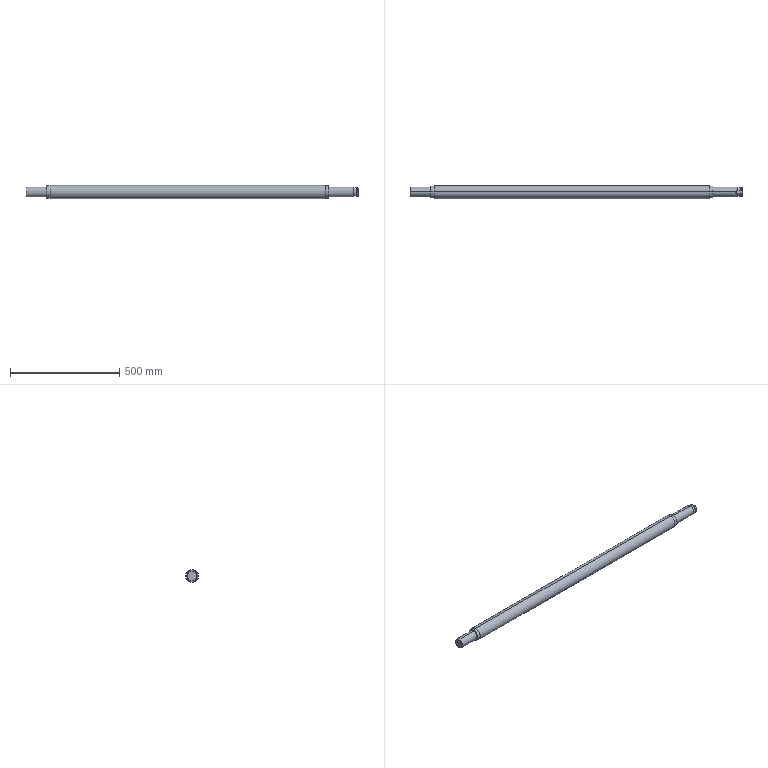Part | SolidWorks | features BaseBody 1 | 1 solid | 33 faces | box 1520 x 60 x 60 mm | volume 3990554 mm3 | cylinder 16 | plane 13 | cone 4 | commonest cylinder face diameters 45 x4 55 x4 12 x2 40 x2 60 x2 36 x1
STEP:
#1=CARTESIAN_POINT('',(3106.374,1848.107,21.685));
#2=VERTEX_POINT('',#1);
#3=CARTESIAN_POINT('',(3100.374,1842.107,22.5));
#4=VERTEX_POINT('',#3);
#5=CARTESIAN_POINT('',(3106.374,1848.107,21.685));
#6=CARTESIAN_POINT('',(3105.976,1848.107,21.685));
#7=CARTESIAN_POINT('',(3105.584,1848.068,21.696));
#8=CARTESIAN_POINT('',(3105.007,1847.953,21.727));
#9=CARTESIAN_POINT('',(3104.816,1847.905,21.74));
#10=CARTESIAN_POINT('',(3104.438,1847.79,21.771));
#11=CARTESIAN_POINT('',(3104.251,1847.723,21.788));
#12=CARTESIAN_POINT('',(3103.707,1847.496,21.846));
#13=CARTESIAN_POINT('',(3103.363,1847.312,21.891));
#14=CARTESIAN_POINT('',(3102.875,1846.985,21.965));
#15=CARTESIAN_POINT('',(3102.716,1846.867,21.991));
#16=CARTESIAN_POINT('',(3102.412,1846.617,22.044));
#17=CARTESIAN_POINT('',(3102.267,1846.486,22.07));
#18=CARTESIAN_POINT('',(3101.854,1846.073,22.15));
#19=CARTESIAN_POINT('',(3101.607,1845.772,22.202));
#20=CARTESIAN_POINT('',(3101.168,1845.116,22.3));
#21=CARTESIAN_POINT('',(3100.983,1844.769,22.345));
#22=CARTESIAN_POINT('',(3100.758,1844.228,22.401));
#23=CARTESIAN_POINT('',(3100.692,1844.044,22.417));
#24=CARTESIAN_POINT('',(3100.577,1843.667,22.447));
#25=CARTESIAN_POINT('',(3100.528,1843.473,22.459));
#26=CARTESIAN_POINT('',(3100.413,1842.892,22.49));
#27=CARTESIAN_POINT('',(3100.374,1842.501,22.5));
#28=CARTESIAN_POINT('',(3100.374,1842.107,22.5));
#29=B_SPLINE_CURVE_WITH_KNOTS('',3,(#5,#6,#7,#8,#9,#10,#11,#12,#13,#14,#15,#16,#17,#18,#19,#20,#21,#22,#23,#24,#25,#26,#27,#28),.UNSPECIFIED.,.F.,.F.,(4,2,2,2,2,2,2,2,2,2,2,4),(0.,0.001178,0.001767,0.002356,0.003534,0.004123,0.004712,0.00589,0.007068,0.007657,0.008246,0.009425),.UNSPECIFIED.);
#30=EDGE_CURVE('',#2,#4,#29,.T.);
#31=ORIENTED_EDGE('',*,*,#30,.T.);
#32=CARTESIAN_POINT('',(3100.374,1842.107,15.));
#33=VERTEX_POINT('',#32);
#34=CARTESIAN_POINT('',(3100.374,1842.107,30.));
#35=DIRECTION('',(0.,0.,-1.));
#36=VECTOR('',#35,1000.);
#37=LINE('',#34,#36);
#38=EDGE_CURVE('',#4,#33,#37,.T.);
#39=ORIENTED_EDGE('',*,*,#38,.T.);
#40=CARTESIAN_POINT('',(3106.374,1848.107,15.));
#41=VERTEX_POINT('',#40);
#42=CARTESIAN_POINT('',(3106.374,1842.107,15.));
#43=DIRECTION('',(0.,0.,1.));
#44=DIRECTION('',(1.,0.,0.));
#45=AXIS2_PLACEMENT_3D('',#42,#43,#44);
#46=CIRCLE('',#45,6.);
#47=EDGE_CURVE('',#41,#33,#46,.T.);
#48=ORIENTED_EDGE('',*,*,#47,.F.);
#49=CARTESIAN_POINT('',(3106.374,1848.107,30.));
#50=DIRECTION('',(0.,0.,-1.));
#51=VECTOR('',#50,1000.);
#52=LINE('',#49,#51);
#53=EDGE_CURVE('',#2,#41,#52,.T.);
#54=ORIENTED_EDGE('',*,*,#53,.F.);
#55=EDGE_LOOP('',(#31,#39,#48,#54));
#56=FACE_OUTER_BOUND('',#55,.T.);
#57=CARTESIAN_POINT('',(3106.374,1842.107,30.));
#58=DIRECTION('',(0.,0.,-1.));
#59=DIRECTION('',(-1.,0.,0.));
#60=AXIS2_PLACEMENT_3D('',#57,#58,#59);
#61=CYLINDRICAL_SURFACE('',#60,6.);
#62=ADVANCED_FACE('',(#56),#61,.F.);
#63=CARTESIAN_POINT('',(2993.374,1842.107,27.5));
#64=VERTEX_POINT('',#63);
#65=CARTESIAN_POINT('',(2993.374,1842.107,-27.5));
#66=VERTEX_POINT('',#65);
#67=CARTESIAN_POINT('',(2993.374,1842.107,0.));
#68=DIRECTION('',(-1.,0.,0.));
#69=DIRECTION('',(0.,0.,1.));
#70=AXIS2_PLACEMENT_3D('',#67,#68,#69);
#71=CIRCLE('',#70,27.5);
#72=EDGE_CURVE('',#64,#66,#71,.T.);
#73=ORIENTED_EDGE('',*,*,#72,.T.);
#74=CARTESIAN_POINT('',(2978.374,1842.107,-27.5));
#75=VERTEX_POINT('',#74);
#76=CARTESIAN_POINT('',(1599.374,1842.107,-27.5));
#77=DIRECTION('',(-1.,0.,0.));
#78=VECTOR('',#77,1000.);
#79=LINE('',#76,#78);
#80=EDGE_CURVE('',#66,#75,#79,.T.);
#81=ORIENTED_EDGE('',*,*,#80,.T.);
#82=CARTESIAN_POINT('',(2978.374,1842.107,27.5));
#83=VERTEX_POINT('',#82);
#84=CARTESIAN_POINT('',(2978.374,1842.107,0.));
#85=DIRECTION('',(-1.,0.,0.));
#86=DIRECTION('',(0.,0.,1.));
#87=AXIS2_PLACEMENT_3D('',#84,#85,#86);
#88=CIRCLE('',#87,27.5);
#89=EDGE_CURVE('',#83,#75,#88,.T.);
#90=ORIENTED_EDGE('',*,*,#89,.F.);
#91=CARTESIAN_POINT('',(1599.374,1842.107,27.5));
#92=DIRECTION('',(-1.,0.,0.));
#93=VECTOR('',#92,1000.);
#94=LINE('',#91,#93);
#95=EDGE_CURVE('',#64,#83,#94,.T.);
#96=ORIENTED_EDGE('',*,*,#95,.F.);
#97=EDGE_LOOP('',(#73,#81,#90,#96));
#98=FACE_OUTER_BOUND('',#97,.T.);
#99=CARTESIAN_POINT('',(1599.374,1842.107,0.));
#100=DIRECTION('',(-1.,0.,0.));
#101=DIRECTION('',(0.,0.,1.));
#102=AXIS2_PLACEMENT_3D('',#99,#100,#101);
#103=CYLINDRICAL_SURFACE('',#102,27.5);
#104=ADVANCED_FACE('',(#98),#103,.T.);
#105=CARTESIAN_POINT('',(2978.374,1842.107,30.));
#106=VERTEX_POINT('',#105);
#107=CARTESIAN_POINT('',(2978.374,1842.107,-30.));
#108=VERTEX_POINT('',#107);
#109=CARTESIAN_POINT('',(2978.374,1842.107,0.));
#110=DIRECTION('',(-1.,0.,0.));
#111=DIRECTION('',(0.,0.,1.));
#112=AXIS2_PLACEMENT_3D('',#109,#110,#111);
#113=CIRCLE('',#112,30.);
#114=EDGE_CURVE('',#106,#108,#113,.T.);
#115=ORIENTED_EDGE('',*,*,#114,.T.);
#116=CARTESIAN_POINT('',(1718.374,1842.107,-30.));
#117=VERTEX_POINT('',#116);
#118=CARTESIAN_POINT('',(1599.374,1842.107,-30.));
#119=DIRECTION('',(-1.,0.,0.));
#120=VECTOR('',#119,1000.);
#121=LINE('',#118,#120);
#122=EDGE_CURVE('',#108,#117,#121,.T.);
#123=ORIENTED_EDGE('',*,*,#122,.T.);
#124=CARTESIAN_POINT('',(1718.374,1842.107,30.));
#125=VERTEX_POINT('',#124);
#126=CARTESIAN_POINT('',(1718.374,1842.107,0.));
#127=DIRECTION('',(-1.,0.,0.));
#128=DIRECTION('',(0.,0.,1.));
#129=AXIS2_PLACEMENT_3D('',#126,#127,#128);
#130=CIRCLE('',#129,30.);
#131=EDGE_CURVE('',#125,#117,#130,.T.);
#132=ORIENTED_EDGE('',*,*,#131,.F.);
#133=CARTESIAN_POINT('',(1599.374,1842.107,30.));
#134=DIRECTION('',(-1.,0.,0.));
#135=VECTOR('',#134,1000.);
#136=LINE('',#133,#135);
#137=EDGE_CURVE('',#106,#125,#136,.T.);
#138=ORIENTED_EDGE('',*,*,#137,.F.);
#139=EDGE_LOOP('',(#115,#123,#132,#138));
#140=FACE_OUTER_BOUND('',#139,.T.);
#141=CARTESIAN_POINT('',(1599.374,1842.107,0.));
#142=DIRECTION('',(-1.,0.,0.));
#143=DIRECTION('',(0.,0.,1.));
#144=AXIS2_PLACEMENT_3D('',#141,#142,#143);
#145=CYLINDRICAL_SURFACE('',#144,30.);
#146=ADVANCED_FACE('',(#140),#145,.T.);
#147=CARTESIAN_POINT('',(1718.374,1842.107,27.5));
#148=VERTEX_POINT('',#147);
#149=CARTESIAN_POINT('',(1718.374,1842.107,-27.5));
#150=VERTEX_POINT('',#149);
#151=CARTESIAN_POINT('',(1718.374,1842.107,0.));
#152=DIRECTION('',(-1.,0.,0.));
#153=DIRECTION('',(0.,0.,1.));
#154=AXIS2_PLACEMENT_3D('',#151,#152,#153);
#155=CIRCLE('',#154,27.5);
#156=EDGE_CURVE('',#148,#150,#155,.T.);
#157=ORIENTED_EDGE('',*,*,#156,.T.);
#158=CARTESIAN_POINT('',(1703.374,1842.107,-27.5));
#159=VERTEX_POINT('',#158);
#160=CARTESIAN_POINT('',(1599.374,1842.107,-27.5));
#161=DIRECTION('',(-1.,0.,0.));
#162=VECTOR('',#161,1000.);
#163=LINE('',#160,#162);
#164=EDGE_CURVE('',#150,#159,#163,.T.);
#165=ORIENTED_EDGE('',*,*,#164,.T.);
#166=CARTESIAN_POINT('',(1703.374,1842.107,27.5));
#167=VERTEX_POINT('',#166);
#168=CARTESIAN_POINT('',(1703.374,1842.107,0.));
#169=DIRECTION('',(-1.,0.,0.));
#170=DIRECTION('',(0.,0.,1.));
#171=AXIS2_PLACEMENT_3D('',#168,#169,#170);
#172=CIRCLE('',#171,27.5);
#173=EDGE_CURVE('',#167,#159,#172,.T.);
#174=ORIENTED_EDGE('',*,*,#173,.F.);
#175=CARTESIAN_POINT('',(1599.374,1842.107,27.5));
#176=DIRECTION('',(-1.,0.,0.));
#177=VECTOR('',#176,1000.);
#178=LINE('',#175,#177);
#179=EDGE_CURVE('',#148,#167,#178,.T.);
#180=ORIENTED_EDGE('',*,*,#179,.F.);
#181=EDGE_LOOP('',(#157,#165,#174,#180));
#182=FACE_OUTER_BOUND('',#181,.T.);
#183=CARTESIAN_POINT('',(1599.374,1842.107,0.));
#184=DIRECTION('',(-1.,0.,0.));
#185=DIRECTION('',(0.,0.,1.));
#186=AXIS2_PLACEMENT_3D('',#183,#184,#185);
#187=CYLINDRICAL_SURFACE('',#186,27.5);
#188=ADVANCED_FACE('',(#182),#187,.T.);
#189=CARTESIAN_POINT('',(1703.374,1842.107,22.5));
#190=VERTEX_POINT('',#189);
#191=CARTESIAN_POINT('',(1703.374,1842.107,-22.5));
#192=VERTEX_POINT('',#191);
#193=CARTESIAN_POINT('',(1703.374,1842.107,0.));
#194=DIRECTION('',(-1.,0.,0.));
#195=DIRECTION('',(0.,0.,1.));
#196=AXIS2_PLACEMENT_3D('',#193,#194,#195);
#197=CIRCLE('',#196,22.5);
#198=EDGE_CURVE('',#190,#192,#197,.T.);
#199=ORIENTED_EDGE('',*,*,#198,.T.);
#200=CARTESIAN_POINT('',(1609.374,1842.107,-22.5));
#201=VERTEX_POINT('',#200);
#202=CARTESIAN_POINT('',(1599.374,1842.107,-22.5));
#203=DIRECTION('',(-1.,0.,0.));
#204=VECTOR('',#203,1000.);
#205=LINE('',#202,#204);
#206=EDGE_CURVE('',#192,#201,#205,.T.);
#207=ORIENTED_EDGE('',*,*,#206,.T.);
#208=CARTESIAN_POINT('',(1609.374,1842.107,22.5));
#209=VERTEX_POINT('',#208);
#210=CARTESIAN_POINT('',(1609.374,1842.107,0.));
#211=DIRECTION('',(-1.,0.,0.));
#212=DIRECTION('',(0.,0.,1.));
#213=AXIS2_PLACEMENT_3D('',#210,#211,#212);
#214=CIRCLE('',#213,22.5);
#215=EDGE_CURVE('',#209,#201,#214,.T.);
#216=ORIENTED_EDGE('',*,*,#215,.F.);
#217=CARTESIAN_POINT('',(1599.374,1842.107,22.5));
#218=DIRECTION('',(-1.,0.,0.));
#219=VECTOR('',#218,1000.);
#220=LINE('',#217,#219);
#221=EDGE_CURVE('',#190,#209,#220,.T.);
#222=ORIENTED_EDGE('',*,*,#221,.F.);
#223=EDGE_LOOP('',(#199,#207,#216,#222));
#224=FACE_OUTER_BOUND('',#223,.T.);
#225=CARTESIAN_POINT('',(1599.374,1842.107,0.));
#226=DIRECTION('',(-1.,0.,0.));
#227=DIRECTION('',(0.,0.,1.));
#228=AXIS2_PLACEMENT_3D('',#225,#226,#227);
#229=CYLINDRICAL_SURFACE('',#228,22.5);
#230=ADVANCED_FACE('',(#224),#229,.T.);
#231=CARTESIAN_POINT('',(1608.374,1842.107,21.5));
#232=VERTEX_POINT('',#231);
#233=CARTESIAN_POINT('',(1608.374,1842.107,-21.5));
#234=VERTEX_POINT('',#233);
#235=CARTESIAN_POINT('',(1608.374,1842.107,0.));
#236=DIRECTION('',(-1.,0.,0.));
#237=DIRECTION('',(0.,0.,1.));
#238=AXIS2_PLACEMENT_3D('',#235,#236,#237);
#239=CIRCLE('',#238,21.5);
#240=EDGE_CURVE('',#232,#234,#239,.T.);
#241=ORIENTED_EDGE('',*,*,#240,.F.);
#242=CARTESIAN_POINT('',(1609.374,1842.107,22.5));
#243=DIRECTION('',(0.7071,0.,0.7071));
#244=VECTOR('',#243,1000.);
#245=LINE('',#242,#244);
#246=EDGE_CURVE('',#232,#209,#245,.T.);
#247=ORIENTED_EDGE('',*,*,#246,.T.);
#248=ORIENTED_EDGE('',*,*,#215,.T.);
#249=CARTESIAN_POINT('',(1609.374,1842.107,-22.5));
#250=DIRECTION('',(0.7071,0.,-0.7071));
#251=VECTOR('',#250,1000.);
#252=LINE('',#249,#251);
#253=EDGE_CURVE('',#234,#201,#252,.T.);
#254=ORIENTED_EDGE('',*,*,#253,.F.);
#255=EDGE_LOOP('',(#241,#247,#248,#254));
#256=FACE_OUTER_BOUND('',#255,.T.);
#257=CARTESIAN_POINT('',(1609.374,1842.107,0.));
#258=DIRECTION('',(1.,0.,0.));
#259=DIRECTION('',(0.,0.,-1.));
#260=AXIS2_PLACEMENT_3D('',#257,#258,#259);
#261=CONICAL_SURFACE('',#260,22.5,0.7854);
#262=ADVANCED_FACE('',(#256),#261,.T.);
#263=CARTESIAN_POINT('',(3107.374,1848.107,21.685));
#264=VERTEX_POINT('',#263);
#265=CARTESIAN_POINT('',(3107.374,1842.107,-22.5));
#266=VERTEX_POINT('',#265);
#267=CARTESIAN_POINT('',(3107.374,1842.107,0.));
#268=DIRECTION('',(-1.,0.,0.));
#269=DIRECTION('',(0.,0.,1.));
#270=AXIS2_PLACEMENT_3D('',#267,#268,#269);
#271=CIRCLE('',#270,22.5);
#272=EDGE_CURVE('',#264,#266,#271,.T.);
#273=ORIENTED_EDGE('',*,*,#272,.T.);
#274=CARTESIAN_POINT('',(2993.374,1842.107,-22.5));
#275=VERTEX_POINT('',#274);
#276=CARTESIAN_POINT('',(1599.374,1842.107,-22.5));
#277=DIRECTION('',(-1.,0.,0.));
#278=VECTOR('',#277,1000.);
#279=LINE('',#276,#278);
#280=EDGE_CURVE('',#266,#275,#279,.T.);
#281=ORIENTED_EDGE('',*,*,#280,.T.);
#282=CARTESIAN_POINT('',(2993.374,1842.107,22.5));
#283=VERTEX_POINT('',#282);
#284=CARTESIAN_POINT('',(2993.374,1842.107,0.));
#285=DIRECTION('',(-1.,0.,0.));
#286=DIRECTION('',(0.,0.,1.));
#287=AXIS2_PLACEMENT_3D('',#284,#285,#286);
#288=CIRCLE('',#287,22.5);
#289=EDGE_CURVE('',#283,#275,#288,.T.);
#290=ORIENTED_EDGE('',*,*,#289,.F.);
#291=CARTESIAN_POINT('',(1599.374,1842.107,22.5));
#292=DIRECTION('',(-1.,0.,0.));
#293=VECTOR('',#292,1000.);
#294=LINE('',#291,#293);
#295=EDGE_CURVE('',#4,#283,#294,.T.);
#296=ORIENTED_EDGE('',*,*,#295,.F.);
#297=ORIENTED_EDGE('',*,*,#30,.F.);
#298=CARTESIAN_POINT('',(1599.374,1848.107,21.685));
#299=DIRECTION('',(-1.,0.,0.));
#300=VECTOR('',#299,1000.);
#301=LINE('',#298,#300);
#302=EDGE_CURVE('',#264,#2,#301,.T.);
#303=ORIENTED_EDGE('',*,*,#302,.F.);
#304=EDGE_LOOP('',(#273,#281,#290,#296,#297,#303));
#305=FACE_OUTER_BOUND('',#304,.T.);
#306=CARTESIAN_POINT('',(1599.374,1842.107,0.));
#307=DIRECTION('',(-1.,0.,0.));
#308=DIRECTION('',(0.,0.,1.));
#309=AXIS2_PLACEMENT_3D('',#306,#307,#308);
#310=CYLINDRICAL_SURFACE('',#309,22.5);
#311=ADVANCED_FACE('',(#305),#310,.T.);
#312=ORIENTED_EDGE('',*,*,#280,.F.);
#313=CARTESIAN_POINT('',(3107.374,1836.107,21.685));
#314=VERTEX_POINT('',#313);
#315=CARTESIAN_POINT('',(3107.374,1842.107,0.));
#316=DIRECTION('',(-1.,0.,0.));
#317=DIRECTION('',(0.,0.,1.));
#318=AXIS2_PLACEMENT_3D('',#315,#316,#317);
#319=CIRCLE('',#318,22.5);
#320=EDGE_CURVE('',#266,#314,#319,.T.);
#321=ORIENTED_EDGE('',*,*,#320,.T.);
#322=CARTESIAN_POINT('',(3106.374,1836.107,21.685));
#323=VERTEX_POINT('',#322);
#324=CARTESIAN_POINT('',(1599.374,1836.107,21.685));
#325=DIRECTION('',(1.,0.,0.));
#326=VECTOR('',#325,1000.);
#327=LINE('',#324,#326);
#328=EDGE_CURVE('',#323,#314,#327,.T.);
#329=ORIENTED_EDGE('',*,*,#328,.F.);
#330=CARTESIAN_POINT('',(3100.374,1842.107,22.5));
#331=CARTESIAN_POINT('',(3100.374,1841.714,22.5));
#332=CARTESIAN_POINT('',(3100.414,1841.315,22.489));
#333=CARTESIAN_POINT('',(3100.568,1840.545,22.449));
#334=CARTESIAN_POINT('',(3100.682,1840.17,22.419));
#335=CARTESIAN_POINT('',(3100.909,1839.624,22.363));
#336=CARTESIAN_POINT('',(3100.994,1839.445,22.343));
#337=CARTESIAN_POINT('',(3101.179,1839.099,22.299));
#338=CARTESIAN_POINT('',(3101.28,1838.932,22.275));
#339=CARTESIAN_POINT('',(3101.496,1838.608,22.227));
#340=CARTESIAN_POINT('',(3101.612,1838.452,22.202));
#341=CARTESIAN_POINT('',(3101.86,1838.15,22.15));
#342=CARTESIAN_POINT('',(3101.993,1838.003,22.123));
#343=CARTESIAN_POINT('',(3102.409,1837.587,22.043));
#344=CARTESIAN_POINT('',(3102.71,1837.34,21.99));
#345=CARTESIAN_POINT('',(3103.358,1836.906,21.892));
#346=CARTESIAN_POINT('',(3103.709,1836.718,21.846));
#347=CARTESIAN_POINT('',(3104.432,1836.417,21.769));
#348=CARTESIAN_POINT('',(3104.805,1836.303,21.739));
#349=CARTESIAN_POINT('',(3105.578,1836.147,21.696));
#350=CARTESIAN_POINT('',(3105.976,1836.107,21.685));
#351=CARTESIAN_POINT('',(3106.374,1836.107,21.685));
#352=B_SPLINE_CURVE_WITH_KNOTS('',3,(#330,#331,#332,#333,#334,#335,#336,#337,#338,#339,#340,#341,#342,#343,#344,#345,#346,#347,#348,#349,#350,#351),.UNSPECIFIED.,.F.,.F.,(4,2,2,2,2,2,2,2,2,2,4),(0.009425,0.0106,0.01178,0.01237,0.01295,0.01354,0.01413,0.01531,0.01648,0.01766,0.01884),.UNSPECIFIED.);
#353=EDGE_CURVE('',#4,#323,#352,.T.);
#354=ORIENTED_EDGE('',*,*,#353,.F.);
#355=ORIENTED_EDGE('',*,*,#295,.T.);
#356=CARTESIAN_POINT('',(2993.374,1842.107,0.));
#357=DIRECTION('',(-1.,0.,0.));
#358=DIRECTION('',(0.,0.,1.));
#359=AXIS2_PLACEMENT_3D('',#356,#357,#358);
#360=CIRCLE('',#359,22.5);
#361=EDGE_CURVE('',#275,#283,#360,.T.);
#362=ORIENTED_EDGE('',*,*,#361,.F.);
#363=EDGE_LOOP('',(#312,#321,#329,#354,#355,#362));
#364=FACE_OUTER_BOUND('',#363,.T.);
#365=CARTESIAN_POINT('',(1599.374,1842.107,0.));
#366=DIRECTION('',(-1.,0.,0.));
#367=DIRECTION('',(0.,0.,1.));
#368=AXIS2_PLACEMENT_3D('',#365,#366,#367);
#369=CYLINDRICAL_SURFACE('',#368,22.5);
#370=ADVANCED_FACE('',(#364),#369,.T.);
#371=CARTESIAN_POINT('',(3108.374,1848.107,20.646));
#372=VERTEX_POINT('',#371);
#373=CARTESIAN_POINT('',(3108.374,1848.107,20.646));
#374=CARTESIAN_POINT('',(3108.041,1848.107,20.993));
#375=CARTESIAN_POINT('',(3107.708,1848.107,21.339));
#376=CARTESIAN_POINT('',(3107.374,1848.107,21.685));
#377=B_SPLINE_CURVE_WITH_KNOTS('',3,(#373,#374,#375,#376),.UNSPECIFIED.,.F.,.F.,(4,4),(0.01106,0.0125),.UNSPECIFIED.);
#378=EDGE_CURVE('',#372,#264,#377,.T.);
#379=ORIENTED_EDGE('',*,*,#378,.F.);
#380=CARTESIAN_POINT('',(3108.374,1836.107,20.646));
#381=VERTEX_POINT('',#380);
#382=CARTESIAN_POINT('',(3108.374,1842.107,0.));
#383=DIRECTION('',(-1.,0.,0.));
#384=DIRECTION('',(0.,0.,1.));
#385=AXIS2_PLACEMENT_3D('',#382,#383,#384);
#386=CIRCLE('',#385,21.5);
#387=EDGE_CURVE('',#372,#381,#386,.T.);
#388=ORIENTED_EDGE('',*,*,#387,.T.);
#389=CARTESIAN_POINT('',(3107.374,1836.107,21.685));
#390=CARTESIAN_POINT('',(3107.708,1836.107,21.339));
#391=CARTESIAN_POINT('',(3108.041,1836.107,20.993));
#392=CARTESIAN_POINT('',(3108.374,1836.107,20.646));
#393=B_SPLINE_CURVE_WITH_KNOTS('',3,(#389,#390,#391,#392),.UNSPECIFIED.,.F.,.F.,(4,4),(0.01085,0.01229),.UNSPECIFIED.);
#394=EDGE_CURVE('',#314,#381,#393,.T.);
#395=ORIENTED_EDGE('',*,*,#394,.F.);
#396=ORIENTED_EDGE('',*,*,#320,.F.);
#397=ORIENTED_EDGE('',*,*,#272,.F.);
#398=EDGE_LOOP('',(#379,#388,#395,#396,#397));
#399=FACE_OUTER_BOUND('',#398,.T.);
#400=CARTESIAN_POINT('',(3108.374,1842.107,0.));
#401=DIRECTION('',(-1.,0.,0.));
#402=DIRECTION('',(0.,0.,1.));
#403=AXIS2_PLACEMENT_3D('',#400,#401,#402);
#404=CONICAL_SURFACE('',#403,21.5,0.7854);
#405=ADVANCED_FACE('',(#399),#404,.T.);
#406=CARTESIAN_POINT('',(3108.374,1848.107,18.329));
#407=VERTEX_POINT('',#406);
#408=CARTESIAN_POINT('',(3108.374,1848.107,0.));
#409=DIRECTION('',(0.,0.,1.));
#410=VECTOR('',#409,1000.);
#411=LINE('',#408,#410);
#412=EDGE_CURVE('',#407,#372,#411,.T.);
#413=ORIENTED_EDGE('',*,*,#412,.F.);
#414=CARTESIAN_POINT('',(3108.374,1836.107,18.329));
#415=VERTEX_POINT('',#414);
#416=CARTESIAN_POINT('',(3108.374,1842.107,0.));
#417=DIRECTION('',(-1.,0.,0.));
#418=DIRECTION('',(0.,0.,1.));
#419=AXIS2_PLACEMENT_3D('',#416,#417,#418);
#420=CIRCLE('',#419,19.286);
#421=EDGE_CURVE('',#407,#415,#420,.T.);
#422=ORIENTED_EDGE('',*,*,#421,.T.);
#423=CARTESIAN_POINT('',(3108.374,1836.107,0.));
#424=DIRECTION('',(0.,0.,-1.));
#425=VECTOR('',#424,1000.);
#426=LINE('',#423,#425);
#427=EDGE_CURVE('',#381,#415,#426,.T.);
#428=ORIENTED_EDGE('',*,*,#427,.F.);
#429=ORIENTED_EDGE('',*,*,#387,.F.);
#430=EDGE_LOOP('',(#413,#422,#428,#429));
#431=FACE_OUTER_BOUND('',#430,.T.);
#432=CARTESIAN_POINT('',(3108.374,1863.607,0.));
#433=DIRECTION('',(-1.,0.,0.));
#434=DIRECTION('',(0.,0.,1.));
#435=AXIS2_PLACEMENT_3D('',#432,#433,#434);
#436=PLANE('',#435);
#437=ADVANCED_FACE('',(#431),#436,.F.);
#438=CARTESIAN_POINT('',(3109.374,1848.107,18.329));
#439=VERTEX_POINT('',#438);
#440=CARTESIAN_POINT('',(1599.374,1848.107,18.329));
#441=DIRECTION('',(-1.,0.,0.));
#442=VECTOR('',#441,1000.);
#443=LINE('',#440,#442);
#444=EDGE_CURVE('',#439,#407,#443,.T.);
#445=ORIENTED_EDGE('',*,*,#444,.F.);
#446=CARTESIAN_POINT('',(3109.374,1836.107,18.329));
#447=VERTEX_POINT('',#446);
#448=CARTESIAN_POINT('',(3109.374,1842.107,0.));
#449=DIRECTION('',(-1.,0.,0.));
#450=DIRECTION('',(0.,0.,1.));
#451=AXIS2_PLACEMENT_3D('',#448,#449,#450);
#452=CIRCLE('',#451,19.286);
#453=EDGE_CURVE('',#439,#447,#452,.T.);
#454=ORIENTED_EDGE('',*,*,#453,.T.);
#455=CARTESIAN_POINT('',(1599.374,1836.107,18.329));
#456=DIRECTION('',(1.,0.,0.));
#457=VECTOR('',#456,1000.);
#458=LINE('',#455,#457);
#459=EDGE_CURVE('',#415,#447,#458,.T.);
#460=ORIENTED_EDGE('',*,*,#459,.F.);
#461=ORIENTED_EDGE('',*,*,#421,.F.);
#462=EDGE_LOOP('',(#445,#454,#460,#461));
#463=FACE_OUTER_BOUND('',#462,.T.);
#464=CARTESIAN_POINT('',(1599.374,1842.107,0.));
#465=DIRECTION('',(-1.,0.,0.));
#466=DIRECTION('',(0.,0.,1.));
#467=AXIS2_PLACEMENT_3D('',#464,#465,#466);
#468=CYLINDRICAL_SURFACE('',#467,19.286);
#469=ADVANCED_FACE('',(#463),#468,.T.);
#470=CARTESIAN_POINT('',(3109.374,1848.107,19.079));
#471=VERTEX_POINT('',#470);
#472=CARTESIAN_POINT('',(3109.374,1848.107,0.));
#473=DIRECTION('',(0.,0.,-1.));
#474=VECTOR('',#473,1000.);
#475=LINE('',#472,#474);
#476=EDGE_CURVE('',#471,#439,#475,.T.);
#477=ORIENTED_EDGE('',*,*,#476,.F.);
#478=CARTESIAN_POINT('',(3109.374,1836.107,19.079));
#479=VERTEX_POINT('',#478);
#480=CARTESIAN_POINT('',(3109.374,1842.107,0.));
#481=DIRECTION('',(-1.,0.,0.));
#482=DIRECTION('',(0.,0.,1.));
#483=AXIS2_PLACEMENT_3D('',#480,#481,#482);
#484=CIRCLE('',#483,20.);
#485=EDGE_CURVE('',#471,#479,#484,.T.);
#486=ORIENTED_EDGE('',*,*,#485,.T.);
#487=CARTESIAN_POINT('',(3109.374,1836.107,0.));
#488=DIRECTION('',(0.,0.,1.));
#489=VECTOR('',#488,1000.);
#490=LINE('',#487,#489);
#491=EDGE_CURVE('',#447,#479,#490,.T.);
#492=ORIENTED_EDGE('',*,*,#491,.F.);
#493=ORIENTED_EDGE('',*,*,#453,.F.);
#494=EDGE_LOOP('',(#477,#486,#492,#493));
#495=FACE_OUTER_BOUND('',#494,.T.);
#496=CARTESIAN_POINT('',(3109.374,1861.393,0.));
#497=DIRECTION('',(1.,0.,0.));
#498=DIRECTION('',(0.,0.,-1.));
#499=AXIS2_PLACEMENT_3D('',#496,#497,#498);
#500=PLANE('',#499);
#501=ADVANCED_FACE('',(#495),#500,.F.);
#502=CARTESIAN_POINT('',(3120.374,1848.107,19.079));
#503=VERTEX_POINT('',#502);
#504=CARTESIAN_POINT('',(1599.374,1848.107,19.079));
#505=DIRECTION('',(-1.,0.,0.));
#506=VECTOR('',#505,1000.);
#507=LINE('',#504,#506);
#508=EDGE_CURVE('',#503,#471,#507,.T.);
#509=ORIENTED_EDGE('',*,*,#508,.F.);
#510=CARTESIAN_POINT('',(3120.374,1836.107,19.079));
#511=VERTEX_POINT('',#510);
#512=CARTESIAN_POINT('',(3120.374,1842.107,0.));
#513=DIRECTION('',(-1.,0.,0.));
#514=DIRECTION('',(0.,0.,1.));
#515=AXIS2_PLACEMENT_3D('',#512,#513,#514);
#516=CIRCLE('',#515,20.);
#517=EDGE_CURVE('',#503,#511,#516,.T.);
#518=ORIENTED_EDGE('',*,*,#517,.T.);
#519=CARTESIAN_POINT('',(1599.374,1836.107,19.079));
#520=DIRECTION('',(1.,0.,0.));
#521=VECTOR('',#520,1000.);
#522=LINE('',#519,#521);
#523=EDGE_CURVE('',#479,#511,#522,.T.);
#524=ORIENTED_EDGE('',*,*,#523,.F.);
#525=ORIENTED_EDGE('',*,*,#485,.F.);
#526=EDGE_LOOP('',(#509,#518,#524,#525));
#527=FACE_OUTER_BOUND('',#526,.T.);
#528=CARTESIAN_POINT('',(1599.374,1842.107,0.));
#529=DIRECTION('',(-1.,0.,0.));
#530=DIRECTION('',(0.,0.,1.));
#531=AXIS2_PLACEMENT_3D('',#528,#529,#530);
#532=CYLINDRICAL_SURFACE('',#531,20.);
#533=ADVANCED_FACE('',(#527),#532,.T.);
#534=CARTESIAN_POINT('',(3120.374,1848.107,16.971));
#535=VERTEX_POINT('',#534);
#536=CARTESIAN_POINT('',(3120.374,1848.107,0.));
#537=DIRECTION('',(0.,0.,1.));
#538=VECTOR('',#537,1000.);
#539=LINE('',#536,#538);
#540=EDGE_CURVE('',#535,#503,#539,.T.);
#541=ORIENTED_EDGE('',*,*,#540,.F.);
#542=CARTESIAN_POINT('',(3120.374,1836.107,16.971));
#543=VERTEX_POINT('',#542);
#544=CARTESIAN_POINT('',(3120.374,1842.107,0.));
#545=DIRECTION('',(-1.,0.,0.));
#546=DIRECTION('',(0.,0.,1.));
#547=AXIS2_PLACEMENT_3D('',#544,#545,#546);
#548=CIRCLE('',#547,18.);
#549=EDGE_CURVE('',#535,#543,#548,.T.);
#550=ORIENTED_EDGE('',*,*,#549,.T.);
#551=CARTESIAN_POINT('',(3120.374,1836.107,0.));
#552=DIRECTION('',(0.,0.,-1.));
#553=VECTOR('',#552,1000.);
#554=LINE('',#551,#553);
#555=EDGE_CURVE('',#511,#543,#554,.T.);
#556=ORIENTED_EDGE('',*,*,#555,.F.);
#557=ORIENTED_EDGE('',*,*,#517,.F.);
#558=EDGE_LOOP('',(#541,#550,#556,#557));
#559=FACE_OUTER_BOUND('',#558,.T.);
#560=CARTESIAN_POINT('',(3120.374,1862.107,0.));
#561=DIRECTION('',(-1.,0.,0.));
#562=DIRECTION('',(0.,0.,1.));
#563=AXIS2_PLACEMENT_3D('',#560,#561,#562);
#564=PLANE('',#563);
#565=ADVANCED_FACE('',(#559),#564,.F.);
#566=CARTESIAN_POINT('',(3122.374,1848.107,16.971));
#567=VERTEX_POINT('',#566);
#568=CARTESIAN_POINT('',(1599.374,1848.107,16.971));
#569=DIRECTION('',(-1.,0.,0.));
#570=VECTOR('',#569,1000.);
#571=LINE('',#568,#570);
#572=EDGE_CURVE('',#567,#535,#571,.T.);
#573=ORIENTED_EDGE('',*,*,#572,.F.);
#574=CARTESIAN_POINT('',(3122.374,1836.107,16.971));
#575=VERTEX_POINT('',#574);
#576=CARTESIAN_POINT('',(3122.374,1842.107,0.));
#577=DIRECTION('',(-1.,0.,0.));
#578=DIRECTION('',(0.,0.,1.));
#579=AXIS2_PLACEMENT_3D('',#576,#577,#578);
#580=CIRCLE('',#579,18.);
#581=EDGE_CURVE('',#567,#575,#580,.T.);
#582=ORIENTED_EDGE('',*,*,#581,.T.);
#583=CARTESIAN_POINT('',(1599.374,1836.107,16.971));
#584=DIRECTION('',(1.,0.,0.));
#585=VECTOR('',#584,1000.);
#586=LINE('',#583,#585);
#587=EDGE_CURVE('',#543,#575,#586,.T.);
#588=ORIENTED_EDGE('',*,*,#587,.F.);
#589=ORIENTED_EDGE('',*,*,#549,.F.);
#590=EDGE_LOOP('',(#573,#582,#588,#589));
#591=FACE_OUTER_BOUND('',#590,.T.);
#592=CARTESIAN_POINT('',(1599.374,1842.107,0.));
#593=DIRECTION('',(-1.,0.,0.));
#594=DIRECTION('',(0.,0.,1.));
#595=AXIS2_PLACEMENT_3D('',#592,#593,#594);
#596=CYLINDRICAL_SURFACE('',#595,18.);
#597=ADVANCED_FACE('',(#591),#596,.T.);
#598=CARTESIAN_POINT('',(3122.374,1848.107,19.079));
#599=VERTEX_POINT('',#598);
#600=CARTESIAN_POINT('',(3122.374,1848.107,0.));
#601=DIRECTION('',(0.,0.,-1.));
#602=VECTOR('',#601,1000.);
#603=LINE('',#600,#602);
#604=EDGE_CURVE('',#599,#567,#603,.T.);
#605=ORIENTED_EDGE('',*,*,#604,.F.);
#606=CARTESIAN_POINT('',(3122.374,1836.107,19.079));
#607=VERTEX_POINT('',#606);
#608=CARTESIAN_POINT('',(3122.374,1842.107,0.));
#609=DIRECTION('',(-1.,0.,0.));
#610=DIRECTION('',(0.,0.,1.));
#611=AXIS2_PLACEMENT_3D('',#608,#609,#610);
#612=CIRCLE('',#611,20.);
#613=EDGE_CURVE('',#599,#607,#612,.T.);
#614=ORIENTED_EDGE('',*,*,#613,.T.);
#615=CARTESIAN_POINT('',(3122.374,1836.107,0.));
#616=DIRECTION('',(0.,0.,1.));
#617=VECTOR('',#616,1000.);
#618=LINE('',#615,#617);
#619=EDGE_CURVE('',#575,#607,#618,.T.);
#620=ORIENTED_EDGE('',*,*,#619,.F.);
#621=ORIENTED_EDGE('',*,*,#581,.F.);
#622=EDGE_LOOP('',(#605,#614,#620,#621));
#623=FACE_OUTER_BOUND('',#622,.T.);
#624=CARTESIAN_POINT('',(3122.374,1860.107,0.));
#625=DIRECTION('',(1.,0.,0.));
#626=DIRECTION('',(0.,0.,-1.));
#627=AXIS2_PLACEMENT_3D('',#624,#625,#626);
#628=PLANE('',#627);
#629=ADVANCED_FACE('',(#623),#628,.F.);
#630=CARTESIAN_POINT('',(3127.374,1848.107,19.079));
#631=VERTEX_POINT('',#630);
#632=CARTESIAN_POINT('',(1599.374,1848.107,19.079));
#633=DIRECTION('',(-1.,0.,0.));
#634=VECTOR('',#633,1000.);
#635=LINE('',#632,#634);
#636=EDGE_CURVE('',#631,#599,#635,.T.);
#637=ORIENTED_EDGE('',*,*,#636,.F.);
#638=CARTESIAN_POINT('',(3127.374,1836.107,19.079));
#639=VERTEX_POINT('',#638);
#640=CARTESIAN_POINT('',(3127.374,1842.107,0.));
#641=DIRECTION('',(-1.,0.,0.));
#642=DIRECTION('',(0.,0.,1.));
#643=AXIS2_PLACEMENT_3D('',#640,#641,#642);
#644=CIRCLE('',#643,20.);
#645=EDGE_CURVE('',#631,#639,#644,.T.);
#646=ORIENTED_EDGE('',*,*,#645,.T.);
#647=CARTESIAN_POINT('',(1599.374,1836.107,19.079));
#648=DIRECTION('',(1.,0.,0.));
#649=VECTOR('',#648,1000.);
#650=LINE('',#647,#649);
#651=EDGE_CURVE('',#607,#639,#650,.T.);
#652=ORIENTED_EDGE('',*,*,#651,.F.);
#653=ORIENTED_EDGE('',*,*,#613,.F.);
#654=EDGE_LOOP('',(#637,#646,#652,#653));
#655=FACE_OUTER_BOUND('',#654,.T.);
#656=CARTESIAN_POINT('',(1599.374,1842.107,0.));
#657=DIRECTION('',(-1.,0.,0.));
#658=DIRECTION('',(0.,0.,1.));
#659=AXIS2_PLACEMENT_3D('',#656,#657,#658);
#660=CYLINDRICAL_SURFACE('',#659,20.);
#661=ADVANCED_FACE('',(#655),#660,.T.);
#662=CARTESIAN_POINT('',(3128.374,1848.107,18.028));
#663=VERTEX_POINT('',#662);
#664=CARTESIAN_POINT('',(3128.374,1848.107,18.028));
#665=CARTESIAN_POINT('',(3128.041,1848.107,18.379));
#666=CARTESIAN_POINT('',(3127.708,1848.107,18.729));
#667=CARTESIAN_POINT('',(3127.374,1848.107,19.079));
#668=B_SPLINE_CURVE_WITH_KNOTS('',3,(#664,#665,#666,#667),.UNSPECIFIED.,.F.,.F.,(4,4),(0.007491,0.008942),.UNSPECIFIED.);
#669=EDGE_CURVE('',#663,#631,#668,.T.);
#670=ORIENTED_EDGE('',*,*,#669,.F.);
#671=CARTESIAN_POINT('',(3128.374,1836.107,18.028));
#672=VERTEX_POINT('',#671);
#673=CARTESIAN_POINT('',(3128.374,1842.107,0.));
#674=DIRECTION('',(-1.,0.,0.));
#675=DIRECTION('',(0.,0.,1.));
#676=AXIS2_PLACEMENT_3D('',#673,#674,#675);
#677=CIRCLE('',#676,19.);
#678=EDGE_CURVE('',#663,#672,#677,.T.);
#679=ORIENTED_EDGE('',*,*,#678,.T.);
#680=CARTESIAN_POINT('',(3127.374,1836.107,19.079));
#681=CARTESIAN_POINT('',(3127.708,1836.107,18.729));
#682=CARTESIAN_POINT('',(3128.041,1836.107,18.379));
#683=CARTESIAN_POINT('',(3128.374,1836.107,18.028));
#684=B_SPLINE_CURVE_WITH_KNOTS('',3,(#680,#681,#682,#683),.UNSPECIFIED.,.F.,.F.,(4,4),(0.007349,0.0088),.UNSPECIFIED.);
#685=EDGE_CURVE('',#639,#672,#684,.T.);
#686=ORIENTED_EDGE('',*,*,#685,.F.);
#687=ORIENTED_EDGE('',*,*,#645,.F.);
#688=EDGE_LOOP('',(#670,#679,#686,#687));
#689=FACE_OUTER_BOUND('',#688,.T.);
#690=CARTESIAN_POINT('',(3128.374,1842.107,0.));
#691=DIRECTION('',(-1.,0.,0.));
#692=DIRECTION('',(0.,0.,1.));
#693=AXIS2_PLACEMENT_3D('',#690,#691,#692);
#694=CONICAL_SURFACE('',#693,19.,0.7854);
#695=ADVANCED_FACE('',(#689),#694,.T.);
#696=CARTESIAN_POINT('',(3128.374,1848.107,15.));
#697=VERTEX_POINT('',#696);
#698=CARTESIAN_POINT('',(3128.374,1848.107,0.));
#699=DIRECTION('',(0.,0.,1.));
#700=VECTOR('',#699,1000.);
#701=LINE('',#698,#700);
#702=EDGE_CURVE('',#697,#663,#701,.T.);
#703=ORIENTED_EDGE('',*,*,#702,.F.);
#704=CARTESIAN_POINT('',(3128.374,1836.107,15.));
#705=VERTEX_POINT('',#704);
#706=CARTESIAN_POINT('',(3128.374,1861.107,15.));
#707=DIRECTION('',(0.,1.,0.));
#708=VECTOR('',#707,1000.);
#709=LINE('',#706,#708);
#710=EDGE_CURVE('',#705,#697,#709,.T.);
#711=ORIENTED_EDGE('',*,*,#710,.F.);
#712=CARTESIAN_POINT('',(3128.374,1836.107,0.));
#713=DIRECTION('',(0.,0.,-1.));
#714=VECTOR('',#713,1000.);
#715=LINE('',#712,#714);
#716=EDGE_CURVE('',#672,#705,#715,.T.);
#717=ORIENTED_EDGE('',*,*,#716,.F.);
#718=ORIENTED_EDGE('',*,*,#678,.F.);
#719=EDGE_LOOP('',(#703,#711,#717,#718));
#720=FACE_OUTER_BOUND('',#719,.T.);
#721=CARTESIAN_POINT('',(3128.374,1861.107,0.));
#722=DIRECTION('',(-1.,0.,0.));
#723=DIRECTION('',(0.,0.,1.));
#724=AXIS2_PLACEMENT_3D('',#721,#722,#723);
#725=PLANE('',#724);
#726=ADVANCED_FACE('',(#720),#725,.F.);
#727=CARTESIAN_POINT('',(1608.374,1842.107,0.));
#728=DIRECTION('',(-1.,0.,0.));
#729=DIRECTION('',(0.,0.,1.));
#730=AXIS2_PLACEMENT_3D('',#727,#728,#729);
#731=CIRCLE('',#730,21.5);
#732=EDGE_CURVE('',#234,#232,#731,.T.);
#733=ORIENTED_EDGE('',*,*,#732,.T.);
#734=ORIENTED_EDGE('',*,*,#240,.T.);
#735=EDGE_LOOP('',(#733,#734));
#736=FACE_OUTER_BOUND('',#735,.T.);
#737=CARTESIAN_POINT('',(1608.374,1842.107,0.));
#738=DIRECTION('',(1.,0.,0.));
#739=DIRECTION('',(0.,0.,-1.));
#740=AXIS2_PLACEMENT_3D('',#737,#738,#739);
#741=PLANE('',#740);
#742=ADVANCED_FACE('',(#736),#741,.F.);
#743=ORIENTED_EDGE('',*,*,#246,.F.);
#744=ORIENTED_EDGE('',*,*,#732,.F.);
#745=ORIENTED_EDGE('',*,*,#253,.T.);
#746=CARTESIAN_POINT('',(1609.374,1842.107,0.));
#747=DIRECTION('',(-1.,0.,0.));
#748=DIRECTION('',(0.,0.,1.));
#749=AXIS2_PLACEMENT_3D('',#746,#747,#748);
#750=CIRCLE('',#749,22.5);
#751=EDGE_CURVE('',#201,#209,#750,.T.);
#752=ORIENTED_EDGE('',*,*,#751,.T.);
#753=EDGE_LOOP('',(#743,#744,#745,#752));
#754=FACE_OUTER_BOUND('',#753,.T.);
#755=CARTESIAN_POINT('',(1609.374,1842.107,0.));
#756=DIRECTION('',(1.,0.,0.));
#757=DIRECTION('',(0.,0.,-1.));
#758=AXIS2_PLACEMENT_3D('',#755,#756,#757);
#759=CONICAL_SURFACE('',#758,22.5,0.7854);
#760=ADVANCED_FACE('',(#754),#759,.T.);
#761=ORIENTED_EDGE('',*,*,#206,.F.);
#762=CARTESIAN_POINT('',(1703.374,1842.107,0.));
#763=DIRECTION('',(-1.,0.,0.));
#764=DIRECTION('',(0.,0.,1.));
#765=AXIS2_PLACEMENT_3D('',#762,#763,#764);
#766=CIRCLE('',#765,22.5);
#767=EDGE_CURVE('',#192,#190,#766,.T.);
#768=ORIENTED_EDGE('',*,*,#767,.T.);
#769=ORIENTED_EDGE('',*,*,#221,.T.);
#770=ORIENTED_EDGE('',*,*,#751,.F.);
#771=EDGE_LOOP('',(#761,#768,#769,#770));
#772=FACE_OUTER_BOUND('',#771,.T.);
#773=CARTESIAN_POINT('',(1599.374,1842.107,0.));
#774=DIRECTION('',(-1.,0.,0.));
#775=DIRECTION('',(0.,0.,1.));
#776=AXIS2_PLACEMENT_3D('',#773,#774,#775);
#777=CYLINDRICAL_SURFACE('',#776,22.5);
#778=ADVANCED_FACE('',(#772),#777,.T.);
#779=ORIENTED_EDGE('',*,*,#198,.F.);
#780=ORIENTED_EDGE('',*,*,#767,.F.);
#781=EDGE_LOOP('',(#779,#780));
#782=FACE_BOUND('',#781,.T.);
#783=ORIENTED_EDGE('',*,*,#173,.T.);
#784=CARTESIAN_POINT('',(1703.374,1842.107,0.));
#785=DIRECTION('',(-1.,0.,0.));
#786=DIRECTION('',(0.,0.,1.));
#787=AXIS2_PLACEMENT_3D('',#784,#785,#786);
#788=CIRCLE('',#787,27.5);
#789=EDGE_CURVE('',#159,#167,#788,.T.);
#790=ORIENTED_EDGE('',*,*,#789,.T.);
#791=EDGE_LOOP('',(#783,#790));
#792=FACE_OUTER_BOUND('',#791,.T.);
#793=CARTESIAN_POINT('',(1703.374,1864.607,0.));
#794=DIRECTION('',(1.,0.,0.));
#795=DIRECTION('',(0.,0.,-1.));
#796=AXIS2_PLACEMENT_3D('',#793,#794,#795);
#797=PLANE('',#796);
#798=ADVANCED_FACE('',(#782,#792),#797,.F.);
#799=ORIENTED_EDGE('',*,*,#164,.F.);
#800=CARTESIAN_POINT('',(1718.374,1842.107,0.));
#801=DIRECTION('',(-1.,0.,0.));
#802=DIRECTION('',(0.,0.,1.));
#803=AXIS2_PLACEMENT_3D('',#800,#801,#802);
#804=CIRCLE('',#803,27.5);
#805=EDGE_CURVE('',#150,#148,#804,.T.);
#806=ORIENTED_EDGE('',*,*,#805,.T.);
#807=ORIENTED_EDGE('',*,*,#179,.T.);
#808=ORIENTED_EDGE('',*,*,#789,.F.);
#809=EDGE_LOOP('',(#799,#806,#807,#808));
#810=FACE_OUTER_BOUND('',#809,.T.);
#811=CARTESIAN_POINT('',(1599.374,1842.107,0.));
#812=DIRECTION('',(-1.,0.,0.));
#813=DIRECTION('',(0.,0.,1.));
#814=AXIS2_PLACEMENT_3D('',#811,#812,#813);
#815=CYLINDRICAL_SURFACE('',#814,27.5);
#816=ADVANCED_FACE('',(#810),#815,.T.);
#817=ORIENTED_EDGE('',*,*,#156,.F.);
#818=ORIENTED_EDGE('',*,*,#805,.F.);
#819=EDGE_LOOP('',(#817,#818));
#820=FACE_BOUND('',#819,.T.);
#821=ORIENTED_EDGE('',*,*,#131,.T.);
#822=CARTESIAN_POINT('',(1718.374,1842.107,0.));
#823=DIRECTION('',(-1.,0.,0.));
#824=DIRECTION('',(0.,0.,1.));
#825=AXIS2_PLACEMENT_3D('',#822,#823,#824);
#826=CIRCLE('',#825,30.);
#827=EDGE_CURVE('',#117,#125,#826,.T.);
#828=ORIENTED_EDGE('',*,*,#827,.T.);
#829=EDGE_LOOP('',(#821,#828));
#830=FACE_OUTER_BOUND('',#829,.T.);
#831=CARTESIAN_POINT('',(1718.374,1869.607,0.));
#832=DIRECTION('',(1.,0.,0.));
#833=DIRECTION('',(0.,0.,-1.));
#834=AXIS2_PLACEMENT_3D('',#831,#832,#833);
#835=PLANE('',#834);
#836=ADVANCED_FACE('',(#820,#830),#835,.F.);
#837=ORIENTED_EDGE('',*,*,#122,.F.);
#838=CARTESIAN_POINT('',(2978.374,1842.107,0.));
#839=DIRECTION('',(-1.,0.,0.));
#840=DIRECTION('',(0.,0.,1.));
#841=AXIS2_PLACEMENT_3D('',#838,#839,#840);
#842=CIRCLE('',#841,30.);
#843=EDGE_CURVE('',#108,#106,#842,.T.);
#844=ORIENTED_EDGE('',*,*,#843,.T.);
#845=ORIENTED_EDGE('',*,*,#137,.T.);
#846=ORIENTED_EDGE('',*,*,#827,.F.);
#847=EDGE_LOOP('',(#837,#844,#845,#846));
#848=FACE_OUTER_BOUND('',#847,.T.);
#849=CARTESIAN_POINT('',(1599.374,1842.107,0.));
#850=DIRECTION('',(-1.,0.,0.));
#851=DIRECTION('',(0.,0.,1.));
#852=AXIS2_PLACEMENT_3D('',#849,#850,#851);
#853=CYLINDRICAL_SURFACE('',#852,30.);
#854=ADVANCED_FACE('',(#848),#853,.T.);
#855=ORIENTED_EDGE('',*,*,#114,.F.);
#856=ORIENTED_EDGE('',*,*,#843,.F.);
#857=EDGE_LOOP('',(#855,#856));
#858=FACE_OUTER_BOUND('',#857,.T.);
#859=ORIENTED_EDGE('',*,*,#89,.T.);
#860=CARTESIAN_POINT('',(2978.374,1842.107,0.));
#861=DIRECTION('',(-1.,0.,0.));
#862=DIRECTION('',(0.,0.,1.));
#863=AXIS2_PLACEMENT_3D('',#860,#861,#862);
#864=CIRCLE('',#863,27.5);
#865=EDGE_CURVE('',#75,#83,#864,.T.);
#866=ORIENTED_EDGE('',*,*,#865,.T.);
#867=EDGE_LOOP('',(#859,#866));
#868=FACE_BOUND('',#867,.T.);
#869=CARTESIAN_POINT('',(2978.374,1872.107,0.));
#870=DIRECTION('',(-1.,0.,0.));
#871=DIRECTION('',(0.,0.,1.));
#872=AXIS2_PLACEMENT_3D('',#869,#870,#871);
#873=PLANE('',#872);
#874=ADVANCED_FACE('',(#858,#868),#873,.F.);
#875=ORIENTED_EDGE('',*,*,#80,.F.);
#876=CARTESIAN_POINT('',(2993.374,1842.107,0.));
#877=DIRECTION('',(-1.,0.,0.));
#878=DIRECTION('',(0.,0.,1.));
#879=AXIS2_PLACEMENT_3D('',#876,#877,#878);
#880=CIRCLE('',#879,27.5);
#881=EDGE_CURVE('',#66,#64,#880,.T.);
#882=ORIENTED_EDGE('',*,*,#881,.T.);
#883=ORIENTED_EDGE('',*,*,#95,.T.);
#884=ORIENTED_EDGE('',*,*,#865,.F.);
#885=EDGE_LOOP('',(#875,#882,#883,#884));
#886=FACE_OUTER_BOUND('',#885,.T.);
#887=CARTESIAN_POINT('',(1599.374,1842.107,0.));
#888=DIRECTION('',(-1.,0.,0.));
#889=DIRECTION('',(0.,0.,1.));
#890=AXIS2_PLACEMENT_3D('',#887,#888,#889);
#891=CYLINDRICAL_SURFACE('',#890,27.5);
#892=ADVANCED_FACE('',(#886),#891,.T.);
#893=ORIENTED_EDGE('',*,*,#72,.F.);
#894=ORIENTED_EDGE('',*,*,#881,.F.);
#895=EDGE_LOOP('',(#893,#894));
#896=FACE_OUTER_BOUND('',#895,.T.);
#897=ORIENTED_EDGE('',*,*,#289,.T.);
#898=ORIENTED_EDGE('',*,*,#361,.T.);
#899=EDGE_LOOP('',(#897,#898));
#900=FACE_BOUND('',#899,.T.);
#901=CARTESIAN_POINT('',(2993.374,1869.607,0.));
#902=DIRECTION('',(-1.,0.,0.));
#903=DIRECTION('',(0.,0.,1.));
#904=AXIS2_PLACEMENT_3D('',#901,#902,#903);
#905=PLANE('',#904);
#906=ADVANCED_FACE('',(#896,#900),#905,.F.);
#907=ORIENTED_EDGE('',*,*,#38,.F.);
#908=ORIENTED_EDGE('',*,*,#353,.T.);
#909=CARTESIAN_POINT('',(3106.374,1836.107,15.));
#910=VERTEX_POINT('',#909);
#911=CARTESIAN_POINT('',(3106.374,1836.107,30.));
#912=DIRECTION('',(0.,0.,-1.));
#913=VECTOR('',#912,1000.);
#914=LINE('',#911,#913);
#915=EDGE_CURVE('',#323,#910,#914,.T.);
#916=ORIENTED_EDGE('',*,*,#915,.T.);
#917=CARTESIAN_POINT('',(3106.374,1842.107,15.));
#918=DIRECTION('',(0.,0.,1.));
#919=DIRECTION('',(1.,0.,0.));
#920=AXIS2_PLACEMENT_3D('',#917,#918,#919);
#921=CIRCLE('',#920,6.);
#922=EDGE_CURVE('',#33,#910,#921,.T.);
#923=ORIENTED_EDGE('',*,*,#922,.F.);
#924=EDGE_LOOP('',(#907,#908,#916,#923));
#925=FACE_OUTER_BOUND('',#924,.T.);
#926=CARTESIAN_POINT('',(3106.374,1842.107,30.));
#927=DIRECTION('',(0.,0.,-1.));
#928=DIRECTION('',(-1.,0.,0.));
#929=AXIS2_PLACEMENT_3D('',#926,#927,#928);
#930=CYLINDRICAL_SURFACE('',#929,6.);
#931=ADVANCED_FACE('',(#925),#930,.F.);
#932=ORIENTED_EDGE('',*,*,#302,.T.);
#933=ORIENTED_EDGE('',*,*,#53,.T.);
#934=CARTESIAN_POINT('',(3128.374,1848.107,15.));
#935=DIRECTION('',(-1.,0.,0.));
#936=VECTOR('',#935,1000.);
#937=LINE('',#934,#936);
#938=EDGE_CURVE('',#697,#41,#937,.T.);
#939=ORIENTED_EDGE('',*,*,#938,.F.);
#940=ORIENTED_EDGE('',*,*,#702,.T.);
#941=ORIENTED_EDGE('',*,*,#669,.T.);
#942=ORIENTED_EDGE('',*,*,#636,.T.);
#943=ORIENTED_EDGE('',*,*,#604,.T.);
#944=ORIENTED_EDGE('',*,*,#572,.T.);
#945=ORIENTED_EDGE('',*,*,#540,.T.);
#946=ORIENTED_EDGE('',*,*,#508,.T.);
#947=ORIENTED_EDGE('',*,*,#476,.T.);
#948=ORIENTED_EDGE('',*,*,#444,.T.);
#949=ORIENTED_EDGE('',*,*,#412,.T.);
#950=ORIENTED_EDGE('',*,*,#378,.T.);
#951=EDGE_LOOP('',(#932,#933,#939,#940,#941,#942,#943,#944,#945,#946,#947,#948,#949,#950));
#952=FACE_OUTER_BOUND('',#951,.T.);
#953=CARTESIAN_POINT('',(3128.374,1848.107,30.));
#954=DIRECTION('',(0.,-1.,0.));
#955=DIRECTION('',(0.,0.,-1.));
#956=AXIS2_PLACEMENT_3D('',#953,#954,#955);
#957=PLANE('',#956);
#958=ADVANCED_FACE('',(#952),#957,.T.);
#959=ORIENTED_EDGE('',*,*,#328,.T.);
#960=ORIENTED_EDGE('',*,*,#394,.T.);
#961=ORIENTED_EDGE('',*,*,#427,.T.);
#962=ORIENTED_EDGE('',*,*,#459,.T.);
#963=ORIENTED_EDGE('',*,*,#491,.T.);
#964=ORIENTED_EDGE('',*,*,#523,.T.);
#965=ORIENTED_EDGE('',*,*,#555,.T.);
#966=ORIENTED_EDGE('',*,*,#587,.T.);
#967=ORIENTED_EDGE('',*,*,#619,.T.);
#968=ORIENTED_EDGE('',*,*,#651,.T.);
#969=ORIENTED_EDGE('',*,*,#685,.T.);
#970=ORIENTED_EDGE('',*,*,#716,.T.);
#971=CARTESIAN_POINT('',(3128.374,1836.107,15.));
#972=DIRECTION('',(1.,0.,0.));
#973=VECTOR('',#972,1000.);
#974=LINE('',#971,#973);
#975=EDGE_CURVE('',#910,#705,#974,.T.);
#976=ORIENTED_EDGE('',*,*,#975,.F.);
#977=ORIENTED_EDGE('',*,*,#915,.F.);
#978=EDGE_LOOP('',(#959,#960,#961,#962,#963,#964,#965,#966,#967,#968,#969,#970,#976,#977));
#979=FACE_OUTER_BOUND('',#978,.T.);
#980=CARTESIAN_POINT('',(3128.374,1836.107,30.));
#981=DIRECTION('',(0.,1.,0.));
#982=DIRECTION('',(0.,0.,1.));
#983=AXIS2_PLACEMENT_3D('',#980,#981,#982);
#984=PLANE('',#983);
#985=ADVANCED_FACE('',(#979),#984,.T.);
#986=ORIENTED_EDGE('',*,*,#710,.T.);
#987=ORIENTED_EDGE('',*,*,#938,.T.);
#988=ORIENTED_EDGE('',*,*,#47,.T.);
#989=ORIENTED_EDGE('',*,*,#922,.T.);
#990=ORIENTED_EDGE('',*,*,#975,.T.);
#991=EDGE_LOOP('',(#986,#987,#988,#989,#990));
#992=FACE_OUTER_BOUND('',#991,.T.);
#993=CARTESIAN_POINT('',(3128.374,1842.107,15.));
#994=DIRECTION('',(0.,0.,1.));
#995=DIRECTION('',(1.,0.,0.));
#996=AXIS2_PLACEMENT_3D('',#993,#994,#995);
#997=PLANE('',#996);
#998=ADVANCED_FACE('',(#992),#997,.T.);
#999=CLOSED_SHELL('',(#62,#104,#146,#188,#230,#262,#311,#370,#405,#437,#469,#501,#533,#565,#597,#629,#661,#695,#726,#742,#760,#778,#798,#816,#836,#854,#874,#892,#906,#931,#958,#985,#998));
#1000=MANIFOLD_SOLID_BREP('',#999);
#1001=CARTESIAN_POINT('',(0.,0.,0.));
#1002=DIRECTION('',(0.,0.,1.));
#1003=DIRECTION('',(1.,0.,0.));
#1004=AXIS2_PLACEMENT_3D('',#1001,#1002,#1003);
#1005=(LENGTH_UNIT()NAMED_UNIT(*)SI_UNIT(.MILLI.,.METRE.));
#1006=UNCERTAINTY_MEASURE_WITH_UNIT(LENGTH_MEASURE(0.00001),#1005,'','');
#1007=(NAMED_UNIT(*)PLANE_ANGLE_UNIT()SI_UNIT($,.RADIAN.));
#1008=(NAMED_UNIT(*)SI_UNIT($,.STERADIAN.)SOLID_ANGLE_UNIT());
#1009=(GEOMETRIC_REPRESENTATION_CONTEXT(3)GLOBAL_UNCERTAINTY_ASSIGNED_CONTEXT((#1006))GLOBAL_UNIT_ASSIGNED_CONTEXT((#1005,#1007,#1008))REPRESENTATION_CONTEXT('',''));
#1010=ADVANCED_BREP_SHAPE_REPRESENTATION('',(#1000,#1004),#1009);